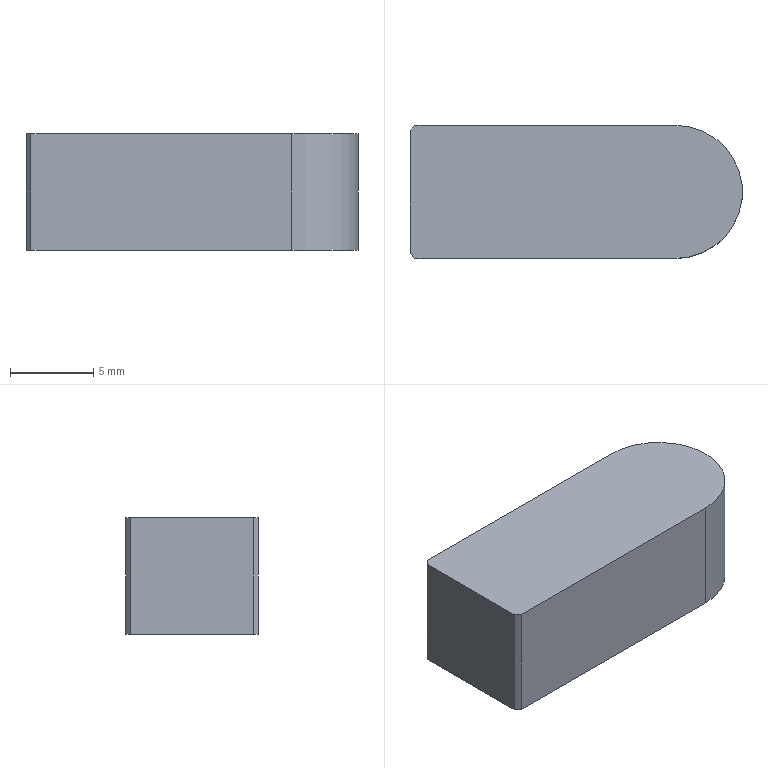Part | STEP file | BLC13-B8-L20^Magnetic powder brake assembly | 1 solid | 8 faces | box 20 x 8 x 7 mm | volume 1071 mm3 | plane 7 | cylinder 1 | commonest cylinder face diameters 8 x1
STEP:
#1=CARTESIAN_POINT('',(0.,0.,0.));
#2=DIRECTION('',(0.,0.,1.));
#3=DIRECTION('',(1.,0.,0.));
#4=AXIS2_PLACEMENT_3D('',#1,#2,#3);
#5=CARTESIAN_POINT('',(-10.,-3.7,0.));
#6=VERTEX_POINT('',#5);
#7=CARTESIAN_POINT('',(-9.7,-4.,0.));
#8=VERTEX_POINT('',#7);
#9=CARTESIAN_POINT('',(-10.,-3.7,0.));
#10=DIRECTION('',(0.7071,-0.7071,0.));
#11=VECTOR('',#10,1.);
#12=LINE('',#9,#11);
#13=CARTESIAN_POINT('',(-10.,-3.7,7.));
#14=DIRECTION('',(0.7071,0.7071,0.));
#15=DIRECTION('',(0.,0.,-1.));
#16=AXIS2_PLACEMENT_3D('',#13,#14,#15);
#17=PLANE('',#16);
#18=CARTESIAN_POINT('',(7.,0.));
#19=DIRECTION('',(0.,-1.));
#20=VECTOR('',#19,1.);
#21=LINE('',#18,#20);
#22=(GEOMETRIC_REPRESENTATION_CONTEXT(2)PARAMETRIC_REPRESENTATION_CONTEXT()REPRESENTATION_CONTEXT('',''));
#23=DEFINITIONAL_REPRESENTATION('',(#21),#22);
#24=PCURVE('',#17,#23);
#25=CARTESIAN_POINT('',(6.,0.,0.));
#26=DIRECTION('',(0.,0.,1.));
#27=DIRECTION('',(1.,0.,0.));
#28=AXIS2_PLACEMENT_3D('',#25,#26,#27);
#29=PLANE('',#28);
#30=CARTESIAN_POINT('',(-16.,-3.7));
#31=DIRECTION('',(0.7071,-0.7071));
#32=VECTOR('',#31,1.);
#33=LINE('',#30,#32);
#34=(GEOMETRIC_REPRESENTATION_CONTEXT(2)PARAMETRIC_REPRESENTATION_CONTEXT()REPRESENTATION_CONTEXT('',''));
#35=DEFINITIONAL_REPRESENTATION('',(#33),#34);
#36=PCURVE('',#29,#35);
#37=SURFACE_CURVE('',#12,(#24,#36),.PCURVE_S1.);
#38=EDGE_CURVE('',#6,#8,#37,.T.);
#39=ORIENTED_EDGE('',*,*,#38,.T.);
#40=CARTESIAN_POINT('',(-9.7,-4.,7.));
#41=VERTEX_POINT('',#40);
#42=CARTESIAN_POINT('',(-9.7,-4.,7.));
#43=DIRECTION('',(0.,0.,-1.));
#44=VECTOR('',#43,1.);
#45=LINE('',#42,#44);
#46=CARTESIAN_POINT('',(0.,-0.4243));
#47=DIRECTION('',(1.,0.));
#48=VECTOR('',#47,1.);
#49=LINE('',#46,#48);
#50=(GEOMETRIC_REPRESENTATION_CONTEXT(2)PARAMETRIC_REPRESENTATION_CONTEXT()REPRESENTATION_CONTEXT('',''));
#51=DEFINITIONAL_REPRESENTATION('',(#49),#50);
#52=PCURVE('',#17,#51);
#53=CARTESIAN_POINT('',(-9.7,-4.,7.));
#54=DIRECTION('',(0.,1.,0.));
#55=DIRECTION('',(1.,0.,0.));
#56=AXIS2_PLACEMENT_3D('',#53,#54,#55);
#57=PLANE('',#56);
#58=CARTESIAN_POINT('',(0.,0.));
#59=DIRECTION('',(0.,1.));
#60=VECTOR('',#59,1.);
#61=LINE('',#58,#60);
#62=(GEOMETRIC_REPRESENTATION_CONTEXT(2)PARAMETRIC_REPRESENTATION_CONTEXT()REPRESENTATION_CONTEXT('',''));
#63=DEFINITIONAL_REPRESENTATION('',(#61),#62);
#64=PCURVE('',#57,#63);
#65=SURFACE_CURVE('',#45,(#52,#64),.PCURVE_S1.);
#66=EDGE_CURVE('',#41,#8,#65,.T.);
#67=ORIENTED_EDGE('',*,*,#66,.F.);
#68=CARTESIAN_POINT('',(-10.,-3.7,7.));
#69=VERTEX_POINT('',#68);
#70=CARTESIAN_POINT('',(-10.,-3.7,7.));
#71=DIRECTION('',(0.7071,-0.7071,0.));
#72=VECTOR('',#71,1.);
#73=LINE('',#70,#72);
#74=CARTESIAN_POINT('',(0.,0.));
#75=DIRECTION('',(0.,-1.));
#76=VECTOR('',#75,1.);
#77=LINE('',#74,#76);
#78=(GEOMETRIC_REPRESENTATION_CONTEXT(2)PARAMETRIC_REPRESENTATION_CONTEXT()REPRESENTATION_CONTEXT('',''));
#79=DEFINITIONAL_REPRESENTATION('',(#77),#78);
#80=PCURVE('',#17,#79);
#81=CARTESIAN_POINT('',(6.,0.,7.));
#82=DIRECTION('',(0.,0.,1.));
#83=DIRECTION('',(1.,0.,0.));
#84=AXIS2_PLACEMENT_3D('',#81,#82,#83);
#85=PLANE('',#84);
#86=CARTESIAN_POINT('',(-16.,-3.7));
#87=DIRECTION('',(0.7071,-0.7071));
#88=VECTOR('',#87,1.);
#89=LINE('',#86,#88);
#90=(GEOMETRIC_REPRESENTATION_CONTEXT(2)PARAMETRIC_REPRESENTATION_CONTEXT()REPRESENTATION_CONTEXT('',''));
#91=DEFINITIONAL_REPRESENTATION('',(#89),#90);
#92=PCURVE('',#85,#91);
#93=SURFACE_CURVE('',#73,(#80,#92),.PCURVE_S1.);
#94=EDGE_CURVE('',#69,#41,#93,.T.);
#95=ORIENTED_EDGE('',*,*,#94,.F.);
#96=CARTESIAN_POINT('',(-10.,-3.7,7.));
#97=DIRECTION('',(0.,0.,-1.));
#98=VECTOR('',#97,1.);
#99=LINE('',#96,#98);
#100=CARTESIAN_POINT('',(0.,0.));
#101=DIRECTION('',(1.,0.));
#102=VECTOR('',#101,1.);
#103=LINE('',#100,#102);
#104=(GEOMETRIC_REPRESENTATION_CONTEXT(2)PARAMETRIC_REPRESENTATION_CONTEXT()REPRESENTATION_CONTEXT('',''));
#105=DEFINITIONAL_REPRESENTATION('',(#103),#104);
#106=PCURVE('',#17,#105);
#107=CARTESIAN_POINT('',(-10.,3.7,7.));
#108=DIRECTION('',(1.,0.,0.));
#109=DIRECTION('',(0.,1.,0.));
#110=AXIS2_PLACEMENT_3D('',#107,#108,#109);
#111=PLANE('',#110);
#112=CARTESIAN_POINT('',(-7.4,0.));
#113=DIRECTION('',(0.,-1.));
#114=VECTOR('',#113,1.);
#115=LINE('',#112,#114);
#116=(GEOMETRIC_REPRESENTATION_CONTEXT(2)PARAMETRIC_REPRESENTATION_CONTEXT()REPRESENTATION_CONTEXT('',''));
#117=DEFINITIONAL_REPRESENTATION('',(#115),#116);
#118=PCURVE('',#111,#117);
#119=SURFACE_CURVE('',#99,(#106,#118),.PCURVE_S1.);
#120=EDGE_CURVE('',#69,#6,#119,.T.);
#121=ORIENTED_EDGE('',*,*,#120,.T.);
#122=EDGE_LOOP('',(#39,#67,#95,#121));
#123=FACE_BOUND('',#122,.T.);
#124=ADVANCED_FACE('',(#123),#17,.F.);
#125=CARTESIAN_POINT('',(-9.7,4.,0.));
#126=VERTEX_POINT('',#125);
#127=CARTESIAN_POINT('',(-10.,3.7,0.));
#128=VERTEX_POINT('',#127);
#129=CARTESIAN_POINT('',(-9.7,4.,0.));
#130=DIRECTION('',(-0.7071,-0.7071,0.));
#131=VECTOR('',#130,1.);
#132=LINE('',#129,#131);
#133=CARTESIAN_POINT('',(-9.7,4.,7.));
#134=DIRECTION('',(0.7071,-0.7071,0.));
#135=DIRECTION('',(0.,0.,-1.));
#136=AXIS2_PLACEMENT_3D('',#133,#134,#135);
#137=PLANE('',#136);
#138=CARTESIAN_POINT('',(7.,0.));
#139=DIRECTION('',(0.,-1.));
#140=VECTOR('',#139,1.);
#141=LINE('',#138,#140);
#142=(GEOMETRIC_REPRESENTATION_CONTEXT(2)PARAMETRIC_REPRESENTATION_CONTEXT()REPRESENTATION_CONTEXT('',''));
#143=DEFINITIONAL_REPRESENTATION('',(#141),#142);
#144=PCURVE('',#137,#143);
#145=CARTESIAN_POINT('',(-15.7,4.));
#146=DIRECTION('',(-0.7071,-0.7071));
#147=VECTOR('',#146,1.);
#148=LINE('',#145,#147);
#149=(GEOMETRIC_REPRESENTATION_CONTEXT(2)PARAMETRIC_REPRESENTATION_CONTEXT()REPRESENTATION_CONTEXT('',''));
#150=DEFINITIONAL_REPRESENTATION('',(#148),#149);
#151=PCURVE('',#29,#150);
#152=SURFACE_CURVE('',#132,(#144,#151),.PCURVE_S1.);
#153=EDGE_CURVE('',#126,#128,#152,.T.);
#154=ORIENTED_EDGE('',*,*,#153,.T.);
#155=CARTESIAN_POINT('',(-10.,3.7,7.));
#156=VERTEX_POINT('',#155);
#157=CARTESIAN_POINT('',(-10.,3.7,7.));
#158=DIRECTION('',(0.,0.,-1.));
#159=VECTOR('',#158,1.);
#160=LINE('',#157,#159);
#161=CARTESIAN_POINT('',(0.,-0.4243));
#162=DIRECTION('',(1.,0.));
#163=VECTOR('',#162,1.);
#164=LINE('',#161,#163);
#165=(GEOMETRIC_REPRESENTATION_CONTEXT(2)PARAMETRIC_REPRESENTATION_CONTEXT()REPRESENTATION_CONTEXT('',''));
#166=DEFINITIONAL_REPRESENTATION('',(#164),#165);
#167=PCURVE('',#137,#166);
#168=CARTESIAN_POINT('',(0.,0.));
#169=DIRECTION('',(0.,-1.));
#170=VECTOR('',#169,1.);
#171=LINE('',#168,#170);
#172=(GEOMETRIC_REPRESENTATION_CONTEXT(2)PARAMETRIC_REPRESENTATION_CONTEXT()REPRESENTATION_CONTEXT('',''));
#173=DEFINITIONAL_REPRESENTATION('',(#171),#172);
#174=PCURVE('',#111,#173);
#175=SURFACE_CURVE('',#160,(#167,#174),.PCURVE_S1.);
#176=EDGE_CURVE('',#156,#128,#175,.T.);
#177=ORIENTED_EDGE('',*,*,#176,.F.);
#178=CARTESIAN_POINT('',(-9.7,4.,7.));
#179=VERTEX_POINT('',#178);
#180=CARTESIAN_POINT('',(-9.7,4.,7.));
#181=DIRECTION('',(-0.7071,-0.7071,0.));
#182=VECTOR('',#181,1.);
#183=LINE('',#180,#182);
#184=CARTESIAN_POINT('',(0.,0.));
#185=DIRECTION('',(0.,-1.));
#186=VECTOR('',#185,1.);
#187=LINE('',#184,#186);
#188=(GEOMETRIC_REPRESENTATION_CONTEXT(2)PARAMETRIC_REPRESENTATION_CONTEXT()REPRESENTATION_CONTEXT('',''));
#189=DEFINITIONAL_REPRESENTATION('',(#187),#188);
#190=PCURVE('',#137,#189);
#191=CARTESIAN_POINT('',(-15.7,4.));
#192=DIRECTION('',(-0.7071,-0.7071));
#193=VECTOR('',#192,1.);
#194=LINE('',#191,#193);
#195=(GEOMETRIC_REPRESENTATION_CONTEXT(2)PARAMETRIC_REPRESENTATION_CONTEXT()REPRESENTATION_CONTEXT('',''));
#196=DEFINITIONAL_REPRESENTATION('',(#194),#195);
#197=PCURVE('',#85,#196);
#198=SURFACE_CURVE('',#183,(#190,#197),.PCURVE_S1.);
#199=EDGE_CURVE('',#179,#156,#198,.T.);
#200=ORIENTED_EDGE('',*,*,#199,.F.);
#201=CARTESIAN_POINT('',(-9.7,4.,7.));
#202=DIRECTION('',(0.,0.,-1.));
#203=VECTOR('',#202,1.);
#204=LINE('',#201,#203);
#205=CARTESIAN_POINT('',(0.,0.));
#206=DIRECTION('',(1.,0.));
#207=VECTOR('',#206,1.);
#208=LINE('',#205,#207);
#209=(GEOMETRIC_REPRESENTATION_CONTEXT(2)PARAMETRIC_REPRESENTATION_CONTEXT()REPRESENTATION_CONTEXT('',''));
#210=DEFINITIONAL_REPRESENTATION('',(#208),#209);
#211=PCURVE('',#137,#210);
#212=CARTESIAN_POINT('',(6.,4.,7.));
#213=DIRECTION('',(0.,-1.,0.));
#214=DIRECTION('',(0.,0.,-1.));
#215=AXIS2_PLACEMENT_3D('',#212,#213,#214);
#216=PLANE('',#215);
#217=CARTESIAN_POINT('',(0.,-15.7));
#218=DIRECTION('',(1.,0.));
#219=VECTOR('',#218,1.);
#220=LINE('',#217,#219);
#221=(GEOMETRIC_REPRESENTATION_CONTEXT(2)PARAMETRIC_REPRESENTATION_CONTEXT()REPRESENTATION_CONTEXT('',''));
#222=DEFINITIONAL_REPRESENTATION('',(#220),#221);
#223=PCURVE('',#216,#222);
#224=SURFACE_CURVE('',#204,(#211,#223),.PCURVE_S1.);
#225=EDGE_CURVE('',#179,#126,#224,.T.);
#226=ORIENTED_EDGE('',*,*,#225,.T.);
#227=EDGE_LOOP('',(#154,#177,#200,#226));
#228=FACE_BOUND('',#227,.T.);
#229=ADVANCED_FACE('',(#228),#137,.F.);
#230=CARTESIAN_POINT('',(-10.,3.7,0.));
#231=DIRECTION('',(0.,-1.,0.));
#232=VECTOR('',#231,1.);
#233=LINE('',#230,#232);
#234=CARTESIAN_POINT('',(-16.,3.7));
#235=DIRECTION('',(0.,-1.));
#236=VECTOR('',#235,1.);
#237=LINE('',#234,#236);
#238=(GEOMETRIC_REPRESENTATION_CONTEXT(2)PARAMETRIC_REPRESENTATION_CONTEXT()REPRESENTATION_CONTEXT('',''));
#239=DEFINITIONAL_REPRESENTATION('',(#237),#238);
#240=PCURVE('',#29,#239);
#241=CARTESIAN_POINT('',(0.,-7.));
#242=DIRECTION('',(-1.,0.));
#243=VECTOR('',#242,1.);
#244=LINE('',#241,#243);
#245=(GEOMETRIC_REPRESENTATION_CONTEXT(2)PARAMETRIC_REPRESENTATION_CONTEXT()REPRESENTATION_CONTEXT('',''));
#246=DEFINITIONAL_REPRESENTATION('',(#244),#245);
#247=PCURVE('',#111,#246);
#248=SURFACE_CURVE('',#233,(#240,#247),.PCURVE_S1.);
#249=EDGE_CURVE('',#128,#6,#248,.T.);
#250=ORIENTED_EDGE('',*,*,#249,.F.);
#251=ORIENTED_EDGE('',*,*,#153,.F.);
#252=CARTESIAN_POINT('',(6.,4.,0.));
#253=VERTEX_POINT('',#252);
#254=CARTESIAN_POINT('',(6.,4.,0.));
#255=DIRECTION('',(-1.,0.,0.));
#256=VECTOR('',#255,1.);
#257=LINE('',#254,#256);
#258=CARTESIAN_POINT('',(0.,4.));
#259=DIRECTION('',(-1.,0.));
#260=VECTOR('',#259,1.);
#261=LINE('',#258,#260);
#262=(GEOMETRIC_REPRESENTATION_CONTEXT(2)PARAMETRIC_REPRESENTATION_CONTEXT()REPRESENTATION_CONTEXT('',''));
#263=DEFINITIONAL_REPRESENTATION('',(#261),#262);
#264=PCURVE('',#29,#263);
#265=CARTESIAN_POINT('',(7.,0.));
#266=DIRECTION('',(0.,-1.));
#267=VECTOR('',#266,1.);
#268=LINE('',#265,#267);
#269=(GEOMETRIC_REPRESENTATION_CONTEXT(2)PARAMETRIC_REPRESENTATION_CONTEXT()REPRESENTATION_CONTEXT('',''));
#270=DEFINITIONAL_REPRESENTATION('',(#268),#269);
#271=PCURVE('',#216,#270);
#272=SURFACE_CURVE('',#257,(#264,#271),.PCURVE_S1.);
#273=EDGE_CURVE('',#253,#126,#272,.T.);
#274=ORIENTED_EDGE('',*,*,#273,.F.);
#275=CARTESIAN_POINT('',(6.,-4.,0.));
#276=VERTEX_POINT('',#275);
#277=CARTESIAN_POINT('',(6.,0.,0.));
#278=DIRECTION('',(0.,0.,1.));
#279=DIRECTION('',(1.,0.,0.));
#280=AXIS2_PLACEMENT_3D('',#277,#278,#279);
#281=CIRCLE('',#280,4.);
#282=CARTESIAN_POINT('',(0.,0.));
#283=DIRECTION('',(1.,0.));
#284=AXIS2_PLACEMENT_2D('',#282,#283);
#285=CIRCLE('',#284,4.);
#286=(GEOMETRIC_REPRESENTATION_CONTEXT(2)PARAMETRIC_REPRESENTATION_CONTEXT()REPRESENTATION_CONTEXT('',''));
#287=DEFINITIONAL_REPRESENTATION('',(#285),#286);
#288=PCURVE('',#29,#287);
#289=CARTESIAN_POINT('',(6.,0.,7.));
#290=DIRECTION('',(0.,0.,1.));
#291=DIRECTION('',(-1.,0.,0.));
#292=AXIS2_PLACEMENT_3D('',#289,#290,#291);
#293=CYLINDRICAL_SURFACE('',#292,4.);
#294=CARTESIAN_POINT('',(-3.142,-7.));
#295=DIRECTION('',(1.,0.));
#296=VECTOR('',#295,1.);
#297=LINE('',#294,#296);
#298=(GEOMETRIC_REPRESENTATION_CONTEXT(2)PARAMETRIC_REPRESENTATION_CONTEXT()REPRESENTATION_CONTEXT('',''));
#299=DEFINITIONAL_REPRESENTATION('',(#297),#298);
#300=PCURVE('',#293,#299);
#301=SURFACE_CURVE('',#281,(#288,#300),.PCURVE_S1.);
#302=EDGE_CURVE('',#276,#253,#301,.T.);
#303=ORIENTED_EDGE('',*,*,#302,.F.);
#304=CARTESIAN_POINT('',(-9.7,-4.,0.));
#305=DIRECTION('',(1.,0.,0.));
#306=VECTOR('',#305,1.);
#307=LINE('',#304,#306);
#308=CARTESIAN_POINT('',(-15.7,-4.));
#309=DIRECTION('',(1.,0.));
#310=VECTOR('',#309,1.);
#311=LINE('',#308,#310);
#312=(GEOMETRIC_REPRESENTATION_CONTEXT(2)PARAMETRIC_REPRESENTATION_CONTEXT()REPRESENTATION_CONTEXT('',''));
#313=DEFINITIONAL_REPRESENTATION('',(#311),#312);
#314=PCURVE('',#29,#313);
#315=CARTESIAN_POINT('',(0.,7.));
#316=DIRECTION('',(1.,0.));
#317=VECTOR('',#316,1.);
#318=LINE('',#315,#317);
#319=(GEOMETRIC_REPRESENTATION_CONTEXT(2)PARAMETRIC_REPRESENTATION_CONTEXT()REPRESENTATION_CONTEXT('',''));
#320=DEFINITIONAL_REPRESENTATION('',(#318),#319);
#321=PCURVE('',#57,#320);
#322=SURFACE_CURVE('',#307,(#314,#321),.PCURVE_S1.);
#323=EDGE_CURVE('',#8,#276,#322,.T.);
#324=ORIENTED_EDGE('',*,*,#323,.F.);
#325=ORIENTED_EDGE('',*,*,#38,.F.);
#326=EDGE_LOOP('',(#250,#251,#274,#303,#324,#325));
#327=FACE_BOUND('',#326,.T.);
#328=ADVANCED_FACE('',(#327),#29,.F.);
#329=ORIENTED_EDGE('',*,*,#323,.T.);
#330=CARTESIAN_POINT('',(6.,-4.,7.));
#331=VERTEX_POINT('',#330);
#332=CARTESIAN_POINT('',(6.,-4.,7.));
#333=DIRECTION('',(0.,0.,-1.));
#334=VECTOR('',#333,1.);
#335=LINE('',#332,#334);
#336=CARTESIAN_POINT('',(15.7,0.));
#337=DIRECTION('',(0.,1.));
#338=VECTOR('',#337,1.);
#339=LINE('',#336,#338);
#340=(GEOMETRIC_REPRESENTATION_CONTEXT(2)PARAMETRIC_REPRESENTATION_CONTEXT()REPRESENTATION_CONTEXT('',''));
#341=DEFINITIONAL_REPRESENTATION('',(#339),#340);
#342=PCURVE('',#57,#341);
#343=CARTESIAN_POINT('',(1.571,0.));
#344=DIRECTION('',(0.,-1.));
#345=VECTOR('',#344,1.);
#346=LINE('',#343,#345);
#347=(GEOMETRIC_REPRESENTATION_CONTEXT(2)PARAMETRIC_REPRESENTATION_CONTEXT()REPRESENTATION_CONTEXT('',''));
#348=DEFINITIONAL_REPRESENTATION('',(#346),#347);
#349=PCURVE('',#293,#348);
#350=SURFACE_CURVE('',#335,(#342,#349),.PCURVE_S1.);
#351=EDGE_CURVE('',#331,#276,#350,.T.);
#352=ORIENTED_EDGE('',*,*,#351,.F.);
#353=CARTESIAN_POINT('',(-9.7,-4.,7.));
#354=DIRECTION('',(1.,0.,0.));
#355=VECTOR('',#354,1.);
#356=LINE('',#353,#355);
#357=CARTESIAN_POINT('',(0.,0.));
#358=DIRECTION('',(1.,0.));
#359=VECTOR('',#358,1.);
#360=LINE('',#357,#359);
#361=(GEOMETRIC_REPRESENTATION_CONTEXT(2)PARAMETRIC_REPRESENTATION_CONTEXT()REPRESENTATION_CONTEXT('',''));
#362=DEFINITIONAL_REPRESENTATION('',(#360),#361);
#363=PCURVE('',#57,#362);
#364=CARTESIAN_POINT('',(-15.7,-4.));
#365=DIRECTION('',(1.,0.));
#366=VECTOR('',#365,1.);
#367=LINE('',#364,#366);
#368=(GEOMETRIC_REPRESENTATION_CONTEXT(2)PARAMETRIC_REPRESENTATION_CONTEXT()REPRESENTATION_CONTEXT('',''));
#369=DEFINITIONAL_REPRESENTATION('',(#367),#368);
#370=PCURVE('',#85,#369);
#371=SURFACE_CURVE('',#356,(#363,#370),.PCURVE_S1.);
#372=EDGE_CURVE('',#41,#331,#371,.T.);
#373=ORIENTED_EDGE('',*,*,#372,.F.);
#374=ORIENTED_EDGE('',*,*,#66,.T.);
#375=EDGE_LOOP('',(#329,#352,#373,#374));
#376=FACE_BOUND('',#375,.T.);
#377=ADVANCED_FACE('',(#376),#57,.F.);
#378=ORIENTED_EDGE('',*,*,#273,.T.);
#379=ORIENTED_EDGE('',*,*,#225,.F.);
#380=CARTESIAN_POINT('',(6.,4.,7.));
#381=VERTEX_POINT('',#380);
#382=CARTESIAN_POINT('',(6.,4.,7.));
#383=DIRECTION('',(-1.,0.,0.));
#384=VECTOR('',#383,1.);
#385=LINE('',#382,#384);
#386=CARTESIAN_POINT('',(0.,0.));
#387=DIRECTION('',(0.,-1.));
#388=VECTOR('',#387,1.);
#389=LINE('',#386,#388);
#390=(GEOMETRIC_REPRESENTATION_CONTEXT(2)PARAMETRIC_REPRESENTATION_CONTEXT()REPRESENTATION_CONTEXT('',''));
#391=DEFINITIONAL_REPRESENTATION('',(#389),#390);
#392=PCURVE('',#216,#391);
#393=CARTESIAN_POINT('',(0.,4.));
#394=DIRECTION('',(-1.,0.));
#395=VECTOR('',#394,1.);
#396=LINE('',#393,#395);
#397=(GEOMETRIC_REPRESENTATION_CONTEXT(2)PARAMETRIC_REPRESENTATION_CONTEXT()REPRESENTATION_CONTEXT('',''));
#398=DEFINITIONAL_REPRESENTATION('',(#396),#397);
#399=PCURVE('',#85,#398);
#400=SURFACE_CURVE('',#385,(#392,#399),.PCURVE_S1.);
#401=EDGE_CURVE('',#381,#179,#400,.T.);
#402=ORIENTED_EDGE('',*,*,#401,.F.);
#403=CARTESIAN_POINT('',(6.,4.,7.));
#404=DIRECTION('',(0.,0.,-1.));
#405=VECTOR('',#404,1.);
#406=LINE('',#403,#405);
#407=CARTESIAN_POINT('',(0.,0.));
#408=DIRECTION('',(1.,0.));
#409=VECTOR('',#408,1.);
#410=LINE('',#407,#409);
#411=(GEOMETRIC_REPRESENTATION_CONTEXT(2)PARAMETRIC_REPRESENTATION_CONTEXT()REPRESENTATION_CONTEXT('',''));
#412=DEFINITIONAL_REPRESENTATION('',(#410),#411);
#413=PCURVE('',#216,#412);
#414=CARTESIAN_POINT('',(4.712,0.));
#415=DIRECTION('',(0.,-1.));
#416=VECTOR('',#415,1.);
#417=LINE('',#414,#416);
#418=(GEOMETRIC_REPRESENTATION_CONTEXT(2)PARAMETRIC_REPRESENTATION_CONTEXT()REPRESENTATION_CONTEXT('',''));
#419=DEFINITIONAL_REPRESENTATION('',(#417),#418);
#420=PCURVE('',#293,#419);
#421=SURFACE_CURVE('',#406,(#413,#420),.PCURVE_S1.);
#422=EDGE_CURVE('',#381,#253,#421,.T.);
#423=ORIENTED_EDGE('',*,*,#422,.T.);
#424=EDGE_LOOP('',(#378,#379,#402,#423));
#425=FACE_BOUND('',#424,.T.);
#426=ADVANCED_FACE('',(#425),#216,.F.);
#427=ORIENTED_EDGE('',*,*,#302,.T.);
#428=ORIENTED_EDGE('',*,*,#422,.F.);
#429=CARTESIAN_POINT('',(6.,0.,7.));
#430=DIRECTION('',(0.,0.,1.));
#431=DIRECTION('',(1.,0.,0.));
#432=AXIS2_PLACEMENT_3D('',#429,#430,#431);
#433=CIRCLE('',#432,4.);
#434=CARTESIAN_POINT('',(-3.142,0.));
#435=DIRECTION('',(1.,0.));
#436=VECTOR('',#435,1.);
#437=LINE('',#434,#436);
#438=(GEOMETRIC_REPRESENTATION_CONTEXT(2)PARAMETRIC_REPRESENTATION_CONTEXT()REPRESENTATION_CONTEXT('',''));
#439=DEFINITIONAL_REPRESENTATION('',(#437),#438);
#440=PCURVE('',#293,#439);
#441=CARTESIAN_POINT('',(0.,0.));
#442=DIRECTION('',(1.,0.));
#443=AXIS2_PLACEMENT_2D('',#441,#442);
#444=CIRCLE('',#443,4.);
#445=(GEOMETRIC_REPRESENTATION_CONTEXT(2)PARAMETRIC_REPRESENTATION_CONTEXT()REPRESENTATION_CONTEXT('',''));
#446=DEFINITIONAL_REPRESENTATION('',(#444),#445);
#447=PCURVE('',#85,#446);
#448=SURFACE_CURVE('',#433,(#440,#447),.PCURVE_S1.);
#449=EDGE_CURVE('',#331,#381,#448,.T.);
#450=ORIENTED_EDGE('',*,*,#449,.F.);
#451=ORIENTED_EDGE('',*,*,#351,.T.);
#452=EDGE_LOOP('',(#427,#428,#450,#451));
#453=FACE_BOUND('',#452,.T.);
#454=ADVANCED_FACE('',(#453),#293,.T.);
#455=CARTESIAN_POINT('',(-10.,3.7,7.));
#456=DIRECTION('',(0.,-1.,0.));
#457=VECTOR('',#456,1.);
#458=LINE('',#455,#457);
#459=CARTESIAN_POINT('',(-16.,3.7));
#460=DIRECTION('',(0.,-1.));
#461=VECTOR('',#460,1.);
#462=LINE('',#459,#461);
#463=(GEOMETRIC_REPRESENTATION_CONTEXT(2)PARAMETRIC_REPRESENTATION_CONTEXT()REPRESENTATION_CONTEXT('',''));
#464=DEFINITIONAL_REPRESENTATION('',(#462),#463);
#465=PCURVE('',#85,#464);
#466=CARTESIAN_POINT('',(0.,0.));
#467=DIRECTION('',(-1.,0.));
#468=VECTOR('',#467,1.);
#469=LINE('',#466,#468);
#470=(GEOMETRIC_REPRESENTATION_CONTEXT(2)PARAMETRIC_REPRESENTATION_CONTEXT()REPRESENTATION_CONTEXT('',''));
#471=DEFINITIONAL_REPRESENTATION('',(#469),#470);
#472=PCURVE('',#111,#471);
#473=SURFACE_CURVE('',#458,(#465,#472),.PCURVE_S1.);
#474=EDGE_CURVE('',#156,#69,#473,.T.);
#475=ORIENTED_EDGE('',*,*,#474,.T.);
#476=ORIENTED_EDGE('',*,*,#94,.T.);
#477=ORIENTED_EDGE('',*,*,#372,.T.);
#478=ORIENTED_EDGE('',*,*,#449,.T.);
#479=ORIENTED_EDGE('',*,*,#401,.T.);
#480=ORIENTED_EDGE('',*,*,#199,.T.);
#481=EDGE_LOOP('',(#475,#476,#477,#478,#479,#480));
#482=FACE_BOUND('',#481,.T.);
#483=ADVANCED_FACE('',(#482),#85,.T.);
#484=ORIENTED_EDGE('',*,*,#249,.T.);
#485=ORIENTED_EDGE('',*,*,#120,.F.);
#486=ORIENTED_EDGE('',*,*,#474,.F.);
#487=ORIENTED_EDGE('',*,*,#176,.T.);
#488=EDGE_LOOP('',(#484,#485,#486,#487));
#489=FACE_BOUND('',#488,.T.);
#490=ADVANCED_FACE('',(#489),#111,.F.);
#491=CLOSED_SHELL('',(#124,#229,#328,#377,#426,#454,#483,#490));
#492=MANIFOLD_SOLID_BREP('',#491);
#493=(LENGTH_UNIT()NAMED_UNIT(*)SI_UNIT(.MILLI.,.METRE.));
#494=UNCERTAINTY_MEASURE_WITH_UNIT(LENGTH_MEASURE(0.0000001),#493,'','');
#495=(NAMED_UNIT(*)PLANE_ANGLE_UNIT()SI_UNIT($,.RADIAN.));
#496=(NAMED_UNIT(*)SI_UNIT($,.STERADIAN.)SOLID_ANGLE_UNIT());
#497=(GEOMETRIC_REPRESENTATION_CONTEXT(3)GLOBAL_UNCERTAINTY_ASSIGNED_CONTEXT((#494))GLOBAL_UNIT_ASSIGNED_CONTEXT((#493,#495,#496))REPRESENTATION_CONTEXT('',''));
#498=ADVANCED_BREP_SHAPE_REPRESENTATION('',(#4,#492),#497);